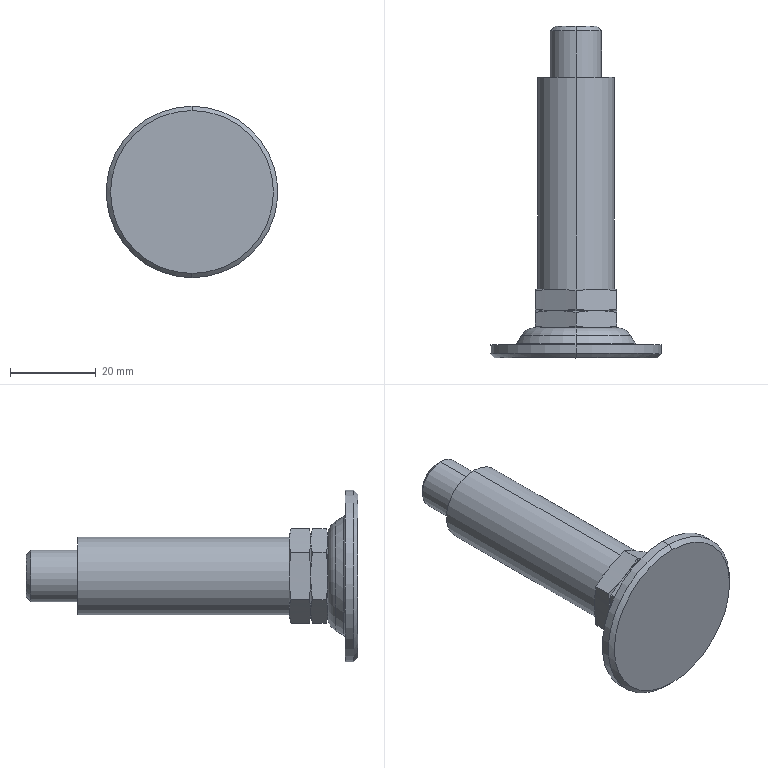Part | SolidWorks | features BaseBody 1 | 1 solid | 62 faces | box 40 x 77.4 x 40 mm | volume 22460 mm3 | cone 34 | plane 18 | cylinder 6 | torus 4 | commonest cylinder face diameters 12 x2 18 x2 40 x2